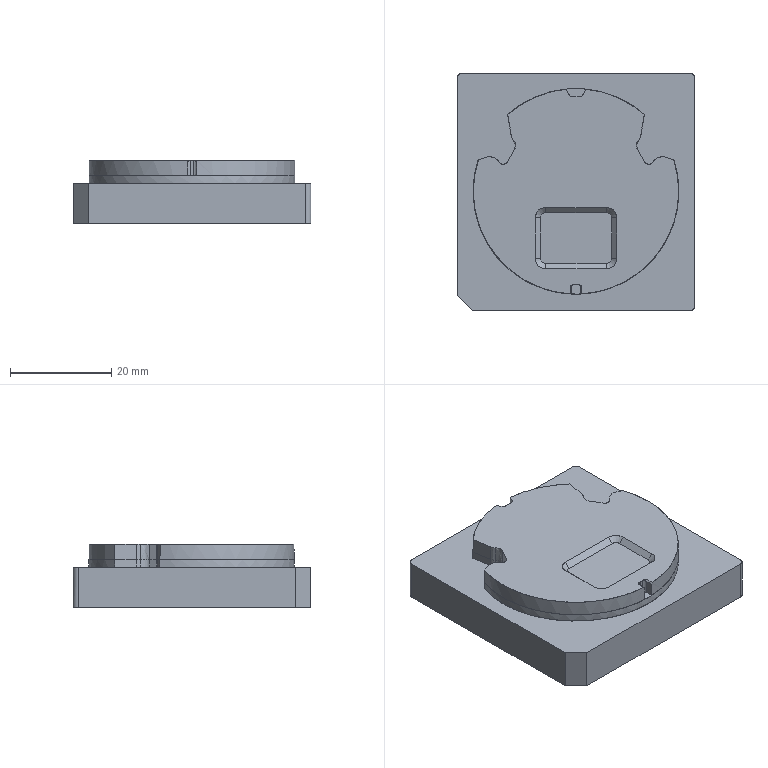NC program | PowerMill | posted with a generic post | part box 47 x 47 x 12.511 mm
Lines 16490 to 17340 of 154620:
N16587 M6
N16588 S8500 M03
N16589 G00 G90 X0.0 Y0.0
N16590 G43 Z11.801 H3
N16591
N16592 G05 P10000 R8
N16593 X8.0731 Y-29.7261
N16594 Z0.8015
N16595 G01 Z-0.3985 F360.0
N16596 X6.7353 Y-24.6236 F600.0
N16597 X25.5562 Y-1.9987
N16598 X25.5883 Y-1.5693
N16599 X25.6315 Y-0.6717
N16600 X25.6393 Y0.5127
N16601 X25.6161 Y1.3031
N16602 X25.5654 Y2.0901
N16603 X25.507 Y2.729
N16604 X25.4367 Y3.3667
N16605 X25.3064 Y4.2643
N16606 X25.2026 Y4.8347
N16607 X0.0682 Y-25.3796
N16608 X-0.0006 Y-25.3643
N16609 X-0.2273 Y-25.4095
N16610 X-0.6653 Y-25.4698
N16611 X-0.9944 Y-25.4892
N16612 X-1.5723 Y-25.4782
N16613 X-2.47 Y-25.4075
N16614 X-3.3639 Y-25.3036
N16615 X-4.3423 Y-25.155
N16616 X-5.1622 Y-25.0019
N16617 X-5.5788 Y-24.9093
N16618 X23.3358 Y9.8491
N16619 X23.1751 Y10.0254
N16620 G03 X22.4624 Y10.6441 I-4.1102 J-4.0148
N16621 G01 X22.1931 Y10.8271
N16622 X21.66 Y11.1242
N16623 X21.2612 Y11.2983
N16624 X19.923 Y11.7874
N16625 X19.2873 Y11.9983
N16626 X19.1237 Y12.0443
N16627 X-10.3228 Y-23.3536
N16628 X-10.8845 Y-23.1012
N16629 X-11.2861 Y-22.9054
N16630 G02 X-12.6859 Y-22.1643 I9.0307 J18.7487
N16631 G01 X-13.0242 Y-21.9728
N16632 X-13.8105 Y-21.4901
N16633 X-14.4546 Y-21.062
N16634 X18.0747 Y18.0418
N16635 X17.9868 Y18.1869
N16636 X17.7674 Y18.499
N16637 X17.6267 Y18.6759
N16638 X17.2761 Y19.0573
N16639 X16.9682 Y19.3425
N16640 X16.2327 Y19.9695
N16641 X15.4796 Y20.5604
N16642 X14.6397 Y21.1711
N16643 X-18.0357 Y-18.1084
N16644 X-18.4776 Y-17.6601
N16645 X-18.8447 Y-17.2753
N16646 X-19.521 Y-16.5123
N16647 X-20.1253 Y-15.7742
N16648 X-20.4187 Y-15.3964
N16649 X-21.0702 Y-14.4976
N16650 X10.5343 Y23.4945
N16651 X9.864 Y23.7878
N16652 X9.076 Y24.0989
N16653 G03 X7.4964 Y24.6369 I-8.7943 J-23.2318
N16654 G01 X6.9537 Y24.7991
N16655 X6.0562 Y25.0349
N16656 X5.8215 Y25.0877
N16657 X-23.4956 Y-10.1547
N16658 X-23.8914 Y-9.1978
N16659 X-24.2219 Y-8.3007
N16660 X-24.5206 Y-7.3872
N16661 X-24.7479 Y-6.6003
N16662 X-24.9306 Y-5.8833
N16663 X-25.094 Y-5.1617
N16664 X-25.1479 Y-4.8824
N16665 X-0.0196 Y25.3246
N16666 X-0.2814 Y25.4155
N16667 X-0.7684 Y25.5466
N16668 X-1.1691 Y25.6186
N16669 X-1.5622 Y25.6593
N16670 X-2.0177 Y25.6692
N16671 X-2.3692 Y25.6506
N16672 X-3.3673 Y25.5391
N16673 X-4.2648 Y25.4039
N16674 X-5.1623 Y25.2358
N16675 X-6.1971 Y25.0009
N16676 X-6.364 Y24.9564
N16677 X-25.5818 Y1.8545
N16678 G00 Z11.801
N16679 G05 P0
N16680 (---------------)
N16681 ( END TOOLPATH : 粗公基准台01-平坦面平行-D10 )
N16682 (---------------)
N16683 ( START TOOLPATH : 粗公基准台01-基准面偏置-D10 )
N16684 (---------------)
N16685 G00 X0.0 Y0.0 Z9.8015
N16686 G05 P10000 R8
N16687 X-1.2909 Y34.125
N16688 Z-3.51
N16689 G01 Z-4.71 F360.0
N16690 Y28.85 F600.0
N16691 X-1.1818 Y25.6576
N16692 X-0.3939 Y25.6845
N16693 X0.3939
N16694 X1.1818 Y25.6576
N16695 X2.3636 Y25.5778
N16696 X2.7576 Y25.5383
N16697 X3.5454 Y25.4406
N16698 X4.3333 Y25.3152
N16699 X5.1212 Y25.169
N16700 X5.9091 Y24.9928
N16701 X6.697 Y24.795
N16702 X7.4848 Y24.565
N16703 X8.2727 Y24.3126
N16704 X9.0606 Y24.0249
N16705 X9.8485 Y23.714
N16706 X10.6363 Y23.3701
N16707 X11.4242 Y22.9939
N16708 X12.4452 Y22.4545
N16709 X13.0 Y22.1321
N16710 X13.7878 Y21.6489
N16711 X14.5757 Y21.1257
N16712 X15.3636 Y20.5579
N16713 X16.1515 Y19.9408
N16714 X16.9394 Y19.2707
N16715 X17.1475 Y19.0837
N16716 X17.3557 Y18.8744
N16717 X17.7272 Y18.4343
N16718 X17.87 Y18.2266
N16719 X21.8704 Y20.8973
N16720 G03 X20.2239 Y22.8078 I-8.5726 J-5.7232
N16721 G01 X20.0052 Y23.0062
N16722 G02 X20.4049 Y24.0413 I0.3996 J0.4404
N16723 G01 X21.6865 Y24.0411
N16724 G02 X23.8622 Y21.9726 I-0.0003 J-2.1789
N16725 G01 X24.0451 Y18.3638
N16726 G02 X23.1666 Y18.1885 I-0.4522 J-0.0229
N16727 G01 X23.0036 Y18.6442
N16728 G03 X21.8704 Y20.8973 I-9.7058 J-3.4701
N16729 G01 X17.87 Y18.2266
N16730 X17.9877 Y18.0554
N16731 X18.1766 Y17.7272
N16732 X18.3644 Y17.3333
N16733 X18.5143 Y16.9394
N16734 X18.642 Y16.4919
N16735 X18.7113 Y16.1515
N16736 X18.7627 Y15.7575
N16737 X18.7844 Y15.3636
N16738 X18.7763 Y14.9697
N16739 X18.739 Y14.5757
N16740 X18.4795 Y13.0837
N16741 G03 X19.1955 Y11.9459 I0.9846 J-0.1746
N16742 G01 X19.303 Y11.9159
N16743 X20.0909 Y11.6481
N16744 X21.2727 Y11.2155
N16745 X21.6666 Y11.041
N16746 X21.9825 Y10.872
N16747 X22.4545 Y10.5632
N16748 X22.8284 Y10.2607
N16749 X23.0354 Y10.0673
N16750 X23.2447 Y9.8485
N16751 X23.5834 Y9.4326
N16752 X23.8317 Y9.0606
N16753 X24.0302 Y8.7043
N16754 X24.2249 Y8.2727
N16755 X24.364 Y7.8788
N16756 X24.4811 Y7.4848
N16757 G02 X24.9051 Y5.9091 I-26.8582 J-8.0709
N16758 G01 X25.0713 Y5.1212
N16759 X25.2167 Y4.3333
N16760 X25.3398 Y3.5454
N16761 X25.4306 Y2.7576
N16762 X25.4991 Y1.9697
N16763 X25.5483 Y1.1818
N16764 X25.5675 Y0.3939
N16765 X25.5606 Y-0.3939
N16766 X25.5352 Y-1.1818
N16767 X25.4852 Y-1.9697
N16768 X25.4044 Y-2.7576
N16769 X25.3036 Y-3.5454
N16770 X25.1805 Y-4.3333
N16771 X25.0259 Y-5.1212
N16772 X24.8181 Y-6.0222
N16773 X24.645 Y-6.697
N16774 X24.415 Y-7.4848
N16775 X24.0302 Y-8.622
N16776 X23.5486 Y-9.8485
N16777 X23.1993 Y-10.6363
N16778 X22.8153 Y-11.4242
N16779 X22.3968 Y-12.2121
N16780 X21.9475 Y-13.0
N16781 X21.4596 Y-13.7878
N16782 X20.8787 Y-14.6442
N16783 X20.3517 Y-15.3636
N16784 X19.7262 Y-16.1515
N16785 X19.0475 Y-16.9394
N16786 X18.3104 Y-17.7272
N16787 X18.0208 Y-18.0154
N16788 X21.4108 Y-21.4208
N16789 G03 X22.5154 Y-20.261 I-21.218 J21.3144
N16790 G01 X23.0039 Y-19.7199
N16791 G02 X24.0451 Y-20.1354 I0.4437 J-0.4006
N16792 G01 X24.0008 Y-21.9051
N16793 G02 X22.3478 Y-23.7484 I-1.9074 J0.0477
N16794 G01 X20.1804 Y-24.04
N16795 G02 X19.7036 Y-23.0054 I-0.0795 J0.5906
N16796 G01 X20.246 Y-22.5201
N16797 G03 X21.4108 Y-21.4208 I-20.0492 J22.4098
N16798 G01 X18.0208 Y-18.0154
N16799 X17.5087 Y-18.5151
N16800 X16.9394 Y-19.036
N16801 G02 X15.6675 Y-20.0909 I-17.2106 J19.4564
N16802 G01 X15.3636 Y-20.3232
N16803 X14.5934 Y-20.8787
N16804 X13.7878 Y-21.4181
N16805 X13.0 Y-21.8997
N16806 X12.0113 Y-22.4545
N16807 X11.4242 Y-22.76
N16808 X10.4009 Y-23.2424
N16809 X9.8485 Y-23.4809
N16810 X9.0606 Y-23.791
N16811 X8.2727 Y-24.078
N16812 X7.4848 Y-24.3311
N16813 X6.697 Y-24.5611
N16814 X5.6606 Y-24.8181
N16815 X5.1212 Y-24.9351
N16816 X4.3333 Y-25.0828
N16817 X3.5454 Y-25.2044
N16818 X2.7576 Y-25.3044
N16819 X1.9697 Y-25.3744
N16820 X1.1818 Y-25.426
N16821 X0.4926 Y-25.4488
N16822 X-0.5909 Y-25.4465
N16823 X-1.1818 Y-25.426
N16824 X-1.9697 Y-25.3744
N16825 X-2.7576 Y-25.3044
N16826 X-3.5454 Y-25.2044
N16827 X-4.3333 Y-25.0828
N16828 X-5.1212 Y-24.9351
N16829 X-5.9091 Y-24.7581
N16830 X-6.697 Y-24.5611
N16831 X-7.4848 Y-24.3311
N16832 X-8.4104 Y-24.0302
N16833 X-9.0606 Y-23.791
N16834 X-9.8485 Y-23.4809
N16835 X-10.4009 Y-23.2424
N16836 X-11.4242 Y-22.76
N16837 X-12.2121 Y-22.3452
N16838 X-13.0 Y-21.8997
N16839 X-13.7878 Y-21.4181
N16840 X-14.5934 Y-20.8787
N16841 X-15.3636 Y-20.3232
N16842 X-16.1515 Y-19.7062
N16843 X-16.5051 Y-19.4107
N16844 X-19.7031 Y-23.0071
N16845 G02 X-20.4418 Y-23.9352 I-0.3947 J-0.4439
N16846 G01 X-21.339 Y-23.2978
N16847 G02 X-21.6728 Y-22.9991 I1.1584 J1.6304
N16848 G01 X-23.8797 Y-20.5262
N16849 G02 X-22.9964 Y-19.7344 I0.4425 J0.3949
N16850 G01 X-22.5145 Y-20.2695
N16851 G03 X-20.2417 Y-22.5281 I21.4841 J19.3462
N16852 G01 X-19.7031 Y-23.0071
N16853 X-16.5051 Y-19.4107
N16854 X-16.9394 Y-19.036
N16855 X-17.7272 Y-18.3074
N16856 X-18.5151 Y-17.5156
N16857 X-19.0475 Y-16.9394
N16858 X-19.7262 Y-16.1515
N16859 X-20.3517 Y-15.3636
N16860 X-20.9272 Y-14.5757
N16861 X-21.4596 Y-13.7878
N16862 X-21.9475 Y-13.0
N16863 X-22.4545 Y-12.1082
N16864 X-22.8153 Y-11.4242
N16865 X-23.2001 Y-10.6363
N16866 X-23.5486 Y-9.8485
N16867 X-24.0302 Y-8.622
N16868 X-24.415 Y-7.4848
N16869 X-24.645 Y-6.697
N16870 X-24.8458 Y-5.9091
N16871 X-25.0259 Y-5.1212
N16872 X-25.1805 Y-4.3333
N16873 X-25.3036 Y-3.5454
N16874 X-25.4044 Y-2.7576
N16875 X-25.4852 Y-1.9697
N16876 X-25.5352 Y-1.1818
N16877 X-25.5606 Y-0.3939
N16878 X-25.5675 Y0.3939
N16879 X-25.5483 Y1.1818
N16880 X-25.4991 Y1.9697
N16881 X-25.4306 Y2.7576
N16882 X-25.3398 Y3.5454
N16883 X-25.2167 Y4.3333
N16884 X-25.072 Y5.1212
N16885 X-24.9051 Y5.9091
N16886 X-24.7081 Y6.697
N16887 X-24.3641 Y7.8788
N16888 X-24.2249 Y8.2727
N16889 X-24.0302 Y8.7043
N16890 X-23.8317 Y9.0606
N16891 X-23.5673 Y9.4545
N16892 X-23.2424 Y9.8508
N16893 X-23.0354 Y10.0673
N16894 X-22.8284 Y10.2607
N16895 X-22.4545 Y10.5632
N16896 X-22.009 Y10.856
N16897 X-21.6666 Y11.041
N16898 X-21.2727 Y11.2155
N16899 X-20.0909 Y11.6481
N16900 X-19.303 Y11.9159
N16901 X-19.1955 Y11.9459
N16902 G03 X-18.4795 Y13.0837 I-0.2686 J0.9632
N16903 G01 X-18.739 Y14.5757
N16904 X-18.7769 Y14.9697
N16905 X-18.7844 Y15.3636
N16906 X-18.7627 Y15.7575
N16907 X-18.7113 Y16.1515
N16908 X-18.6297 Y16.5435
N16909 X-18.5143 Y16.9394
N16910 X-18.3643 Y17.3333
N16911 X-18.1766 Y17.7272
N16912 X-17.9717 Y18.0808
N16913 X-17.8641 Y18.2364
N16914 X-21.8617 Y20.9161
N16915 G03 X-22.9918 Y18.6821 I8.5301 J-5.7179
N16916 G01 X-23.1613 Y18.212
N16917 G02 X-24.0403 Y18.3702 I-0.4261 J0.1536
N16918 G01 X-24.0059 Y21.7785
N16919 G02 X-22.1745 Y23.8303 I2.0887 J-0.0211
N16920 G01 X-20.4792 Y24.0408
N16921 G02 X-20.006 Y23.0082 I0.0734 J-0.5911
N16922 G01 X-20.2246 Y22.8103
N16923 G03 X-21.8617 Y20.9161 I6.8929 J-7.6121
N16924 G01 X-17.8641 Y18.2364
N16925 X-17.6649 Y18.5151
N16926 X-17.3382 Y18.8929
N16927 X-16.9394 Y19.2707
N16928 X-16.1515 Y19.9408
N16929 X-15.3636 Y20.5579
N16930 X-14.5757 Y21.1257
N16931 X-13.7601 Y21.6666
N16932 X-13.0 Y22.1321
N16933 X-12.4452 Y22.4545
N16934 X-11.4242 Y22.9939
N16935 X-10.6363 Y23.3701
N16936 X-9.8485 Y23.714
N16937 X-9.0606 Y24.0249
N16938 X-8.2727 Y24.3126
N16939 X-7.4848 Y24.565
N16940 X-6.61 Y24.8181
N16941 X-5.9091 Y24.9928
N16942 X-5.1212 Y25.169
N16943 X-4.3333 Y25.3152
N16944 X-3.5454 Y25.4406
N16945 X-2.7576 Y25.5383
N16946 X-1.9697 Y25.6083
N16947 X-1.1818 Y25.6576
N16948 X-1.2909 Y28.85
N16949 G00 Z9.8015
N16950 G05 P0
N16951 (---------------)
N16952 ( END TOOLPATH : 粗公基准台01-基准面偏置-D10 )
N16953 (---------------)
N16954 ( START TOOLPATH : 粗公基准台01-外形侧光-D10 )
N16955 (---------------)
N16956 G00 X0.0 Y0.0 Z10.801
N16957 G05 P10000 R8
N16958 X18.8681 Y-17.273
N16959 Z-3.48
N16960 G01 Z-4.68 F360.0
N16961 G03 X17.8071 Y-17.7116 I-0.001 J-1.5 F600.0
N16962 G02 X-1.7036 Y-25.0226 I-17.8071 J17.832
N16963 G02 X-25.1161 Y-1.941 I1.7036 J25.143
N16964 G01 X-25.1796 Y-0.9051
N16965 X-25.2004 Y0.1301
N16966 G02 X-25.091 Y2.4615 I27.907 J-0.1407
N16967 G01 X-24.9726 Y3.4974
N16968 X-24.8103 Y4.5326
N16969 G02 X-23.9673 Y7.9015 I25.8954 J-4.6901
N16970 G02 X-21.0668 Y10.8979 I4.6204 J-1.5705
N16971 G01 X-19.5143 Y11.463
N16972 G02 X-18.1066 Y11.7954 I2.3877 J-6.9657
N16973 G03 X-17.9208 Y12.0516 I-0.0308 J0.2178
N16974 G01 X-18.1209 Y13.1825
N16975 G02 X-18.3649 Y14.5763 I74.5654 J13.7744
N16976 G02 X-16.7028 Y18.9857 I4.8301 J0.6973
N16977 G02 X-15.9257 Y19.6473 I19.907 J-22.596
N16978 G02 X15.1512 Y20.254 I15.9259 J-19.5396
N16979 G01 X15.9273 Y19.646
N16980 G02 X16.938 Y18.7713 I-14.2696 J-17.509
N16981 G02 X18.3643 Y14.5724 I-3.4028 J-3.4977
N16982 G02 X17.9207 Y12.0516 I-140.8393 J23.485
N16983 G03 X18.1066 Y11.7954 I0.2167 J-0.0384
N16984 G02 X19.5179 Y11.4618 I-0.9808 J-7.3019
N16985 G01 X21.0698 Y10.8967
N16986 G02 X24.0494 Y7.6383 I-1.7267 J-4.5705
N16987 G02 X24.8108 Y4.53 I-24.5311 J-7.6563
N16988 G01 X24.973 Y3.4941
N16989 X25.0913 Y2.4589
N16990 G02 X25.2004 Y0.1275 I-27.8014 J-2.4691
N16991 G01 X25.1794 Y-0.9079
N16992 G02 X24.8146 Y-4.275 I-26.303 J1.1464
N16993 G01 X24.6086 Y-5.3103
N16994 G02 X17.8071 Y-17.7116 I-24.6085 J5.4307
N16995 G03 X17.3671 Y-18.7719 I1.06 J-1.0613
N16996 G01 X18.8114 Y-17.2165
N16997 G03 X17.7504 Y-17.6551 I-0.0011 J-1.5
N16998 G02 X-1.6982 Y-24.9427 I-17.7504 J17.7755
N16999 G02 X-25.0363 Y-1.9361 I1.6982 J25.0631
N17000 G02 X-25.1204 Y0.1291 I25.0501 J2.0545
N17001 G02 X-25.0115 Y2.4524 I27.8508 J-0.1405
N17002 G01 X-24.8936 Y3.4851
N17003 X-24.7317 Y4.5177
N17004 G02 X-23.8923 Y7.8736 I25.8509 J-4.6832
N17005 G02 X-21.0394 Y10.8227 I4.5453 J-1.5426
N17006 G01 X-19.4905 Y11.3867
N17007 G02 X-18.0954 Y11.7162 I2.3641 J-6.8905
N17008 G03 X-17.842 Y12.0655 I-0.042 J0.297
N17009 G01 X-18.0421 Y13.1965
N17010 G02 X-18.2854 Y14.5856 I77.4138 J14.278
N17011 G02 X-16.6508 Y18.9249 I4.7504 J0.688
N17012 G02 X-15.8764 Y19.5843 I20.0404 J-22.7523
N17013 G02 X15.1019 Y20.1911 I15.8766 J-19.4768
N17014 G01 X15.8764 Y19.5843
N17015 G02 X16.8801 Y18.716 I-14.3641 J-17.6197
N17016 G02 X18.2854 Y14.5856 I-3.3451 J-3.4424
N17017 G02 X17.842 Y12.0655 I-140.5932 J23.4421
N17018 G03 X18.0954 Y11.7162 I0.2954 J-0.0523
N17019 G02 X19.4905 Y11.3867 I-0.969 J-7.22
N17020 G01 X21.0394 Y10.8227
N17021 G02 X23.9727 Y7.6155 I-1.6963 J-4.4964
N17022 G02 X24.7317 Y4.5177 I-24.4675 J-7.6369
N17023 G01 X24.8935 Y3.4851
N17024 X25.0115 Y2.4524
N17025 G02 X25.1204 Y0.1291 I-27.7441 J-2.4639
N17026 G01 X25.0995 Y-0.9035
N17027 G02 X24.7361 Y-4.2595 I-26.232 J1.1428
N17028 G01 X24.5306 Y-5.2921
N17029 G02 X17.7504 Y-17.6551 I-24.5305 J5.4125
N17030 G03 X17.3103 Y-18.7155 I1.0599 J-1.0614
N17031 G00 Z10.801
N17032 G05 P0
N17033 (---------------)
N17034 ( END TOOLPATH : 粗公基准台01-外形侧光-D10 )
N17035 (---------------)
N17036 ( START TOOLPATH : 粗公基准台01-基准台侧光-D10 )
N17037 (---------------)
N17038 G00 X0.0 Y0.0 Z9.8015
N17039 G05 P10000 R8
N17040 X28.9315 Y-31.5211
N17041 Z-11.41
N17042 G01 Z-12.61 F360.0
N17043 G03 X25.9767 Y-27.4876 I-1.4774 J2.0168 F600.0
N17044 G01 X25.9724 Y-27.4907
N17045 X25.9701 Y-27.4924
N17046 X25.9676 Y-27.494
N17047 X25.5206 Y-27.7738
N17048 X25.518 Y-27.7754
N17049 X25.5152 Y-27.7769
N17050 X25.0683 Y-28.0105
N17051 X25.0648 Y-28.0122
N17052 X25.0613 Y-28.0138
N17053 X24.5181 Y-28.2342
N17054 X24.5152 Y-28.2353
N17055 X24.5123 Y-28.2363
N17056 X24.1615 Y-28.3482
N17057 X24.1589 Y-28.349
N17058 X24.1561 Y-28.3498
N17059 X23.7091 Y-28.4585
N17060 X23.7061 Y-28.4592
N17061 X23.7031 Y-28.4597
N17062 X23.2561 Y-28.5325
N17063 X23.253 Y-28.5329
N17064 X23.25 Y-28.5333
N17065 X22.803 Y-28.5709
N17066 X22.8004 Y-28.5711
N17067 X22.7978 Y-28.5712
N17068 X22.3509 Y-28.58
N17069 X22.3501
N17070 X22.3493
N17071 X-20.5613 Y-28.5796
N17072 X-20.5636
N17073 X-20.5659 Y-28.5795
N17074 X-21.0129 Y-28.554
N17075 X-21.0165 Y-28.5537
N17076 X-21.02 Y-28.5532
N17077 X-21.467 Y-28.4871
N17078 X-21.4706 Y-28.4864
N17079 X-21.4742 Y-28.4857
N17080 X-21.9212 Y-28.3771
N17081 X-21.9246 Y-28.3762
N17082 X-21.928 Y-28.3751
N17083 X-22.3378 Y-28.2358
N17084 X-22.3414 Y-28.2345
N17085 X-22.345 Y-28.233
N17086 X-22.8292 Y-28.0145
N17087 X-22.8327 Y-28.0128
N17088 X-22.8362 Y-28.0109
N17089 X-23.2325 Y-27.7824
N17090 X-23.2362 Y-27.7802
N17091 X-23.2397 Y-27.7777
N17092 X-23.7374 Y-27.4146
N17093 X-23.7398 Y-27.4128
N17094 X-23.7421 Y-27.4109
N17095 X-23.8407 Y-27.3271
N17096 X-23.8424 Y-27.3256
N17097 X-23.844 Y-27.324
N17098 X-24.1924 Y-26.9917
N17099 X-24.1931 Y-26.9911
N17100 X-24.1938 Y-26.9904
N17101 X-26.9904 Y-24.1938
N17102 X-26.9911 Y-24.1931
N17103 X-26.9917 Y-24.1924
N17104 X-27.324 Y-23.844
N17105 X-27.3256 Y-23.8424
N17106 X-27.3271 Y-23.8407
N17107 X-27.4109 Y-23.7421
N17108 X-27.4127 Y-23.74
N17109 X-27.4143 Y-23.7378
N17110 X-27.7446 Y-23.2908
N17111 X-27.7471 Y-23.2873
N17112 X-27.7494 Y-23.2836
N17113 X-28.0106 Y-22.8366
N17114 X-28.0126 Y-22.8331
N17115 X-28.0144 Y-22.8295
N17116 X-28.2182 Y-22.3825
N17117 X-28.2198 Y-22.3789
N17118 X-28.2211 Y-22.3753
N17119 X-28.375 Y-21.9283
N17120 X-28.3761 Y-21.9248
N17121 X-28.3771 Y-21.9212
N17122 X-28.4857 Y-21.4742
N17123 X-28.4864 Y-21.4706
N17124 X-28.4871 Y-21.467
N17125 X-28.5532 Y-21.02
N17126 X-28.5537 Y-21.0165
N17127 X-28.554 Y-21.0129
N17128 X-28.5795 Y-20.5659
N17129 X-28.5796 Y-20.5636
N17130 Y-20.5613
N17131 X-28.58 Y22.3493
N17132 Y22.3501
N17133 Y22.3509
N17134 X-28.5712 Y22.7978
N17135 X-28.5711 Y22.8004
N17136 X-28.5709 Y22.803
N17137 X-28.5333 Y23.25
N17138 X-28.5329 Y23.253
N17139 X-28.5325 Y23.2561
N17140 X-28.4597 Y23.7031
N17141 X-28.4592 Y23.7061
N17142 X-28.4585 Y23.7091
N17143 X-28.3498 Y24.1561
N17144 X-28.349 Y24.1589
N17145 X-28.3482 Y24.1615
N17146 X-28.2363 Y24.5123
N17147 X-28.2353 Y24.5152
N17148 X-28.2342 Y24.5181
N17149 X-28.0138 Y25.0613
N17150 X-28.0123 Y25.0648
N17151 X-28.0106 Y25.0682
N17152 X-27.7841 Y25.503
N17153 X-27.7826 Y25.5058
N17154 X-27.781 Y25.5084
N17155 X-27.494 Y25.9676
N17156 X-27.4924 Y25.97
N17157 X-27.4907 Y25.9724
N17158 X-27.3307 Y26.191
N17159 X-27.3294 Y26.1927
N17160 X-27.328 Y26.1944
N17161 X-27.1407 Y26.4229
N17162 X-27.1397 Y26.4241
N17163 X-27.1386 Y26.4253
N17164 X-26.8789 Y26.7176
N17165 X-26.8774 Y26.7194
N17166 X-26.8757 Y26.721
N17167 X-26.721 Y26.8757
N17168 X-26.7194 Y26.8774
N17169 X-26.7176 Y26.8789
N17170 X-26.4253 Y27.1386
N17171 X-26.4241 Y27.1397
N17172 X-26.4229 Y27.1407
N17173 X-26.1944 Y27.328
N17174 X-26.1927 Y27.3294
N17175 X-26.191 Y27.3307
N17176 X-25.9724 Y27.4907
N17177 X-25.9701 Y27.4924
N17178 X-25.9676 Y27.494
N17179 X-25.5206 Y27.7738
N17180 X-25.518 Y27.7754
N17181 X-25.5152 Y27.7769
N17182 X-25.0683 Y28.0106
N17183 X-25.0651 Y28.0121
N17184 X-25.0619 Y28.0136
N17185 X-24.6149 Y28.1993
N17186 X-24.612 Y28.2005
N17187 X-24.6091 Y28.2015
N17188 X-24.1621 Y28.348
N17189 X-24.1592 Y28.3489
N17190 X-24.1561 Y28.3497
N17191 X-23.7092 Y28.4585
N17192 X-23.7061 Y28.4592
N17193 X-23.7031 Y28.4597
N17194 X-23.2561 Y28.5325
N17195 X-23.2531 Y28.533
N17196 X-23.25 Y28.5333
N17197 X-22.803 Y28.571
N17198 X-22.8004 Y28.5712
N17199 X-22.7978
N17200 X-22.3509 Y28.58
N17201 X-22.3501
N17202 X-22.3493
N17203 X0.0
N17204 X22.3493
N17205 X22.3501
N17206 X22.3509
N17207 X22.7978 Y28.5712
N17208 X22.8004
N17209 X22.803 Y28.571
N17210 X23.25 Y28.5333
N17211 X23.2531 Y28.533
N17212 X23.2561 Y28.5325
N17213 X23.7031 Y28.4597
N17214 X23.7061 Y28.4592
N17215 X23.7092 Y28.4585
N17216 X24.1561 Y28.3497
N17217 X24.1589 Y28.349
N17218 X24.1615 Y28.3482
N17219 X24.5123 Y28.2363
N17220 X24.5152 Y28.2353
N17221 X24.5181 Y28.2342
N17222 X25.0613 Y28.0138
N17223 X25.0648 Y28.0123
N17224 X25.0682 Y28.0106
N17225 X25.503 Y27.7841
N17226 X25.5058 Y27.7826
N17227 X25.5084 Y27.781
N17228 X25.9676 Y27.494
N17229 X25.97 Y27.4924
N17230 X25.9724 Y27.4907
N17231 X26.191 Y27.3307
N17232 X26.1927 Y27.3294
N17233 X26.1944 Y27.328
N17234 X26.4229 Y27.1407
N17235 X26.4241 Y27.1397
N17236 X26.4253 Y27.1386
N17237 X26.7176 Y26.8789
N17238 X26.7194 Y26.8774
N17239 X26.721 Y26.8757
N17240 X26.8757 Y26.721
N17241 X26.8774 Y26.7194
N17242 X26.8789 Y26.7176
N17243 X27.1386 Y26.4253
N17244 X27.1397 Y26.4241
N17245 X27.1407 Y26.4229
N17246 X27.328 Y26.1944
N17247 X27.3294 Y26.1927
N17248 X27.3307 Y26.191
N17249 X27.4907 Y25.9724
N17250 X27.4924 Y25.9701
N17251 X27.494 Y25.9676
N17252 X27.7738 Y25.5206
N17253 X27.7754 Y25.518
N17254 X27.7769 Y25.5152
N17255 X28.0106 Y25.0683
N17256 X28.0121 Y25.0651
N17257 X28.0135 Y25.0619
N17258 X28.1993 Y24.6149
N17259 X28.2005 Y24.612
N17260 X28.2015 Y24.6091
N17261 X28.348 Y24.1621
N17262 X28.349 Y24.1592
N17263 X28.3498 Y24.1561
N17264 X28.4585 Y23.7091
N17265 X28.4592 Y23.7061
N17266 X28.4597 Y23.7031
N17267 X28.5325 Y23.2561
N17268 X28.5329 Y23.253
N17269 X28.5333 Y23.25
N17270 X28.5709 Y22.803
N17271 X28.5711 Y22.8004
N17272 X28.5712 Y22.7978
N17273 X28.58 Y22.3509
N17274 Y22.3501
N17275 Y22.3493
N17276 Y0.0
N17277 Y-22.3493
N17278 Y-22.3501
N17279 Y-22.3509
N17280 X28.5712 Y-22.7978
N17281 X28.5711 Y-22.8004
N17282 X28.571 Y-22.803
N17283 X28.5333 Y-23.25
N17284 X28.5329 Y-23.2531
N17285 X28.5325 Y-23.2561
N17286 X28.4597 Y-23.7031
N17287 X28.4592 Y-23.7061
N17288 X28.4585 Y-23.7091
N17289 X28.3498 Y-24.1561
N17290 X28.349 Y-24.1589
N17291 X28.3482 Y-24.1615
N17292 X28.2363 Y-24.5123
N17293 X28.2353 Y-24.5152
N17294 X28.2342 Y-24.5181
N17295 X28.0138 Y-25.0613
N17296 X28.0123 Y-25.0648
N17297 X28.0106 Y-25.0682
N17298 X27.7841 Y-25.503
N17299 X27.7826 Y-25.5058
N17300 X27.781 Y-25.5084
N17301 X27.494 Y-25.9676
N17302 X27.4924 Y-25.97
N17303 X27.4907 Y-25.9724
N17304 X27.3307 Y-26.191
N17305 X27.3294 Y-26.1927
N17306 X27.328 Y-26.1944
N17307 X27.1407 Y-26.4229
N17308 X27.1397 Y-26.4241
N17309 X27.1386 Y-26.4253
N17310 X26.8789 Y-26.7176
N17311 X26.8774 Y-26.7194
N17312 X26.8757 Y-26.721
N17313 X26.721 Y-26.8757
N17314 X26.7194 Y-26.8774
N17315 X26.7176 Y-26.8789
N17316 X26.4253 Y-27.1386
N17317 X26.4241 Y-27.1397
N17318 X26.4229 Y-27.1407
N17319 X26.1944 Y-27.328
N17320 X26.1927 Y-27.3294
N17321 X26.191 Y-27.3307
N17322 X25.9767 Y-27.4876
N17323 G03 X28.931 Y-31.5215 I1.4771 J-2.0169
N17324 G01 X28.8843 Y-31.4565
N17325 G03 X25.9253 Y-27.4261 I-1.4795 J2.0152
N17326 G01 X25.9252 Y-27.4262
N17327 X25.4782 Y-27.706
N17328 X25.0312 Y-27.9396
N17329 X24.488 Y-28.1601
N17330 X24.1372 Y-28.272
N17331 X23.6902 Y-28.3808
N17332 X23.2433 Y-28.4536
N17333 X22.7963 Y-28.4912
N17334 X22.3493 Y-28.5
N17335 X-20.5613 Y-28.4996
N17336 X-21.0083 Y-28.4741
N17337 X-21.4553 Y-28.4079
N17338 X-21.9023 Y-28.2993
N17339 X-22.3121 Y-28.1601
N17340 X-22.7963 Y-27.9416
N17341 X-23.1925 Y-27.7131
N17342 X-23.6902 Y-27.35
N17343 X-23.7888 Y-27.2661
N17344 X-24.1372 Y-26.9339
N17345 X-26.9339 Y-24.1372
N17346 X-27.2661 Y-23.7888
N17347 X-27.35 Y-23.6902
N17348 X-27.6803 Y-23.2433
N17349 X-27.9416 Y-22.7963
N17350 X-28.1455 Y-22.3493
N17351 X-28.2993 Y-21.9023
N17352 X-28.4079 Y-21.4553
N17353 X-28.4741 Y-21.0083
N17354 X-28.4996 Y-20.5613
N17355 X-28.5 Y22.3493
N17356 X-28.4912 Y22.7963
N17357 X-28.4536 Y23.2433
N17358 X-28.3808 Y23.6902
N17359 X-28.272 Y24.1372
N17360 X-28.1601 Y24.488
N17361 X-27.9396 Y25.0312
N17362 X-27.7131 Y25.466
N17363 X-27.4262 Y25.9252
N17364 X-27.2661 Y26.1437
N17365 X-27.0788 Y26.3722
N17366 X-26.8191 Y26.6645
N17367 X-26.6645 Y26.8191
N17368 X-26.3722 Y27.0788
N17369 X-26.1437 Y27.2661
N17370 X-25.9252 Y27.4262
N17371 X-25.4782 Y27.706
N17372 X-25.0312 Y27.9397
N17373 X-24.5842 Y28.1255
N17374 X-24.1372 Y28.272
N17375 X-23.6902 Y28.3808
N17376 X-23.2433 Y28.4536
N17377 X-22.7963 Y28.4913
N17378 X-22.3493 Y28.5
N17379 X0.0
N17380 X22.3493
N17381 X22.7963 Y28.4913
N17382 X23.2433 Y28.4536
N17383 X23.6902 Y28.3808
N17384 X24.1372 Y28.272
N17385 X24.488 Y28.1601
N17386 X25.0312 Y27.9397
N17387 X25.466 Y27.7131
N17388 X25.9252 Y27.4262
N17389 X26.1437 Y27.2661
N17390 X26.3722 Y27.0788
N17391 X26.6645 Y26.8191
N17392 X26.8191 Y26.6645
N17393 X27.0788 Y26.3722
N17394 X27.2661 Y26.1437
N17395 X27.4262 Y25.9252
N17396 X27.706 Y25.4782
N17397 X27.9397 Y25.0312
N17398 X28.1255 Y24.5842
N17399 X28.272 Y24.1372
N17400 X28.3808 Y23.6902
N17401 X28.4536 Y23.2433
N17402 X28.4912 Y22.7963
N17403 X28.5 Y22.3493
N17404 Y0.0
N17405 Y-22.3493
N17406 X28.4912 Y-22.7963
N17407 X28.4536 Y-23.2433
N17408 X28.3808 Y-23.6902
N17409 X28.272 Y-24.1372
N17410 X28.1601 Y-24.488
N17411 X27.9396 Y-25.0312
N17412 X27.7131 Y-25.466
N17413 X27.4262 Y-25.9252
N17414 X27.2661 Y-26.1437
N17415 X27.0788 Y-26.3722
N17416 X26.8191 Y-26.6645
N17417 X26.6645 Y-26.8191
N17418 X26.3722 Y-27.0788
N17419 X26.1437 Y-27.2661
N17420 X25.9253 Y-27.4261
N17421 G03 X28.8797 Y-31.4599 I1.4772 J-2.0169
N17422 G00 Z9.8015
N17423 G05 P0
N17424 (---------------)
N17425 ( END TOOLPATH : 粗公基准台01-基准台侧光-D10 )
N17426 (---------------)
N17427
N17428 M05
N17429 G53 Z0.0
N17430 (---------------)
N17431 ( START TOOLPATH : 粗公精光01-等高-D4 )
N17432 (---------------)
N17433 ( TOOL NO.    :14 )
N17434 ( TOOL TYPE   : ENDMILL)
N17435 ( TOOL ID     : D4_2_1)
N17436 ( TOOL DIA    : 4.0 LENGTH 59.56)
N17437 T14